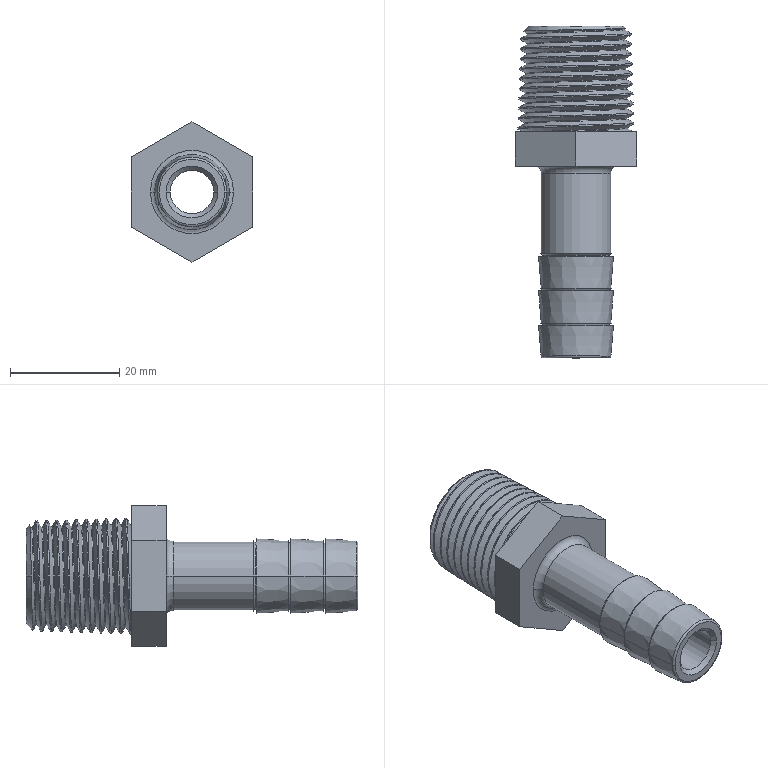Part | SolidWorks | 1 solid | 74 faces | box 22.25 x 60.757 x 25.693 mm | volume 8431 mm3 | cone 36 | torus 16 | plane 13 | cylinder 6 | spline 3 | commonest cylinder face diameters 12.7 x4 7.95 x2